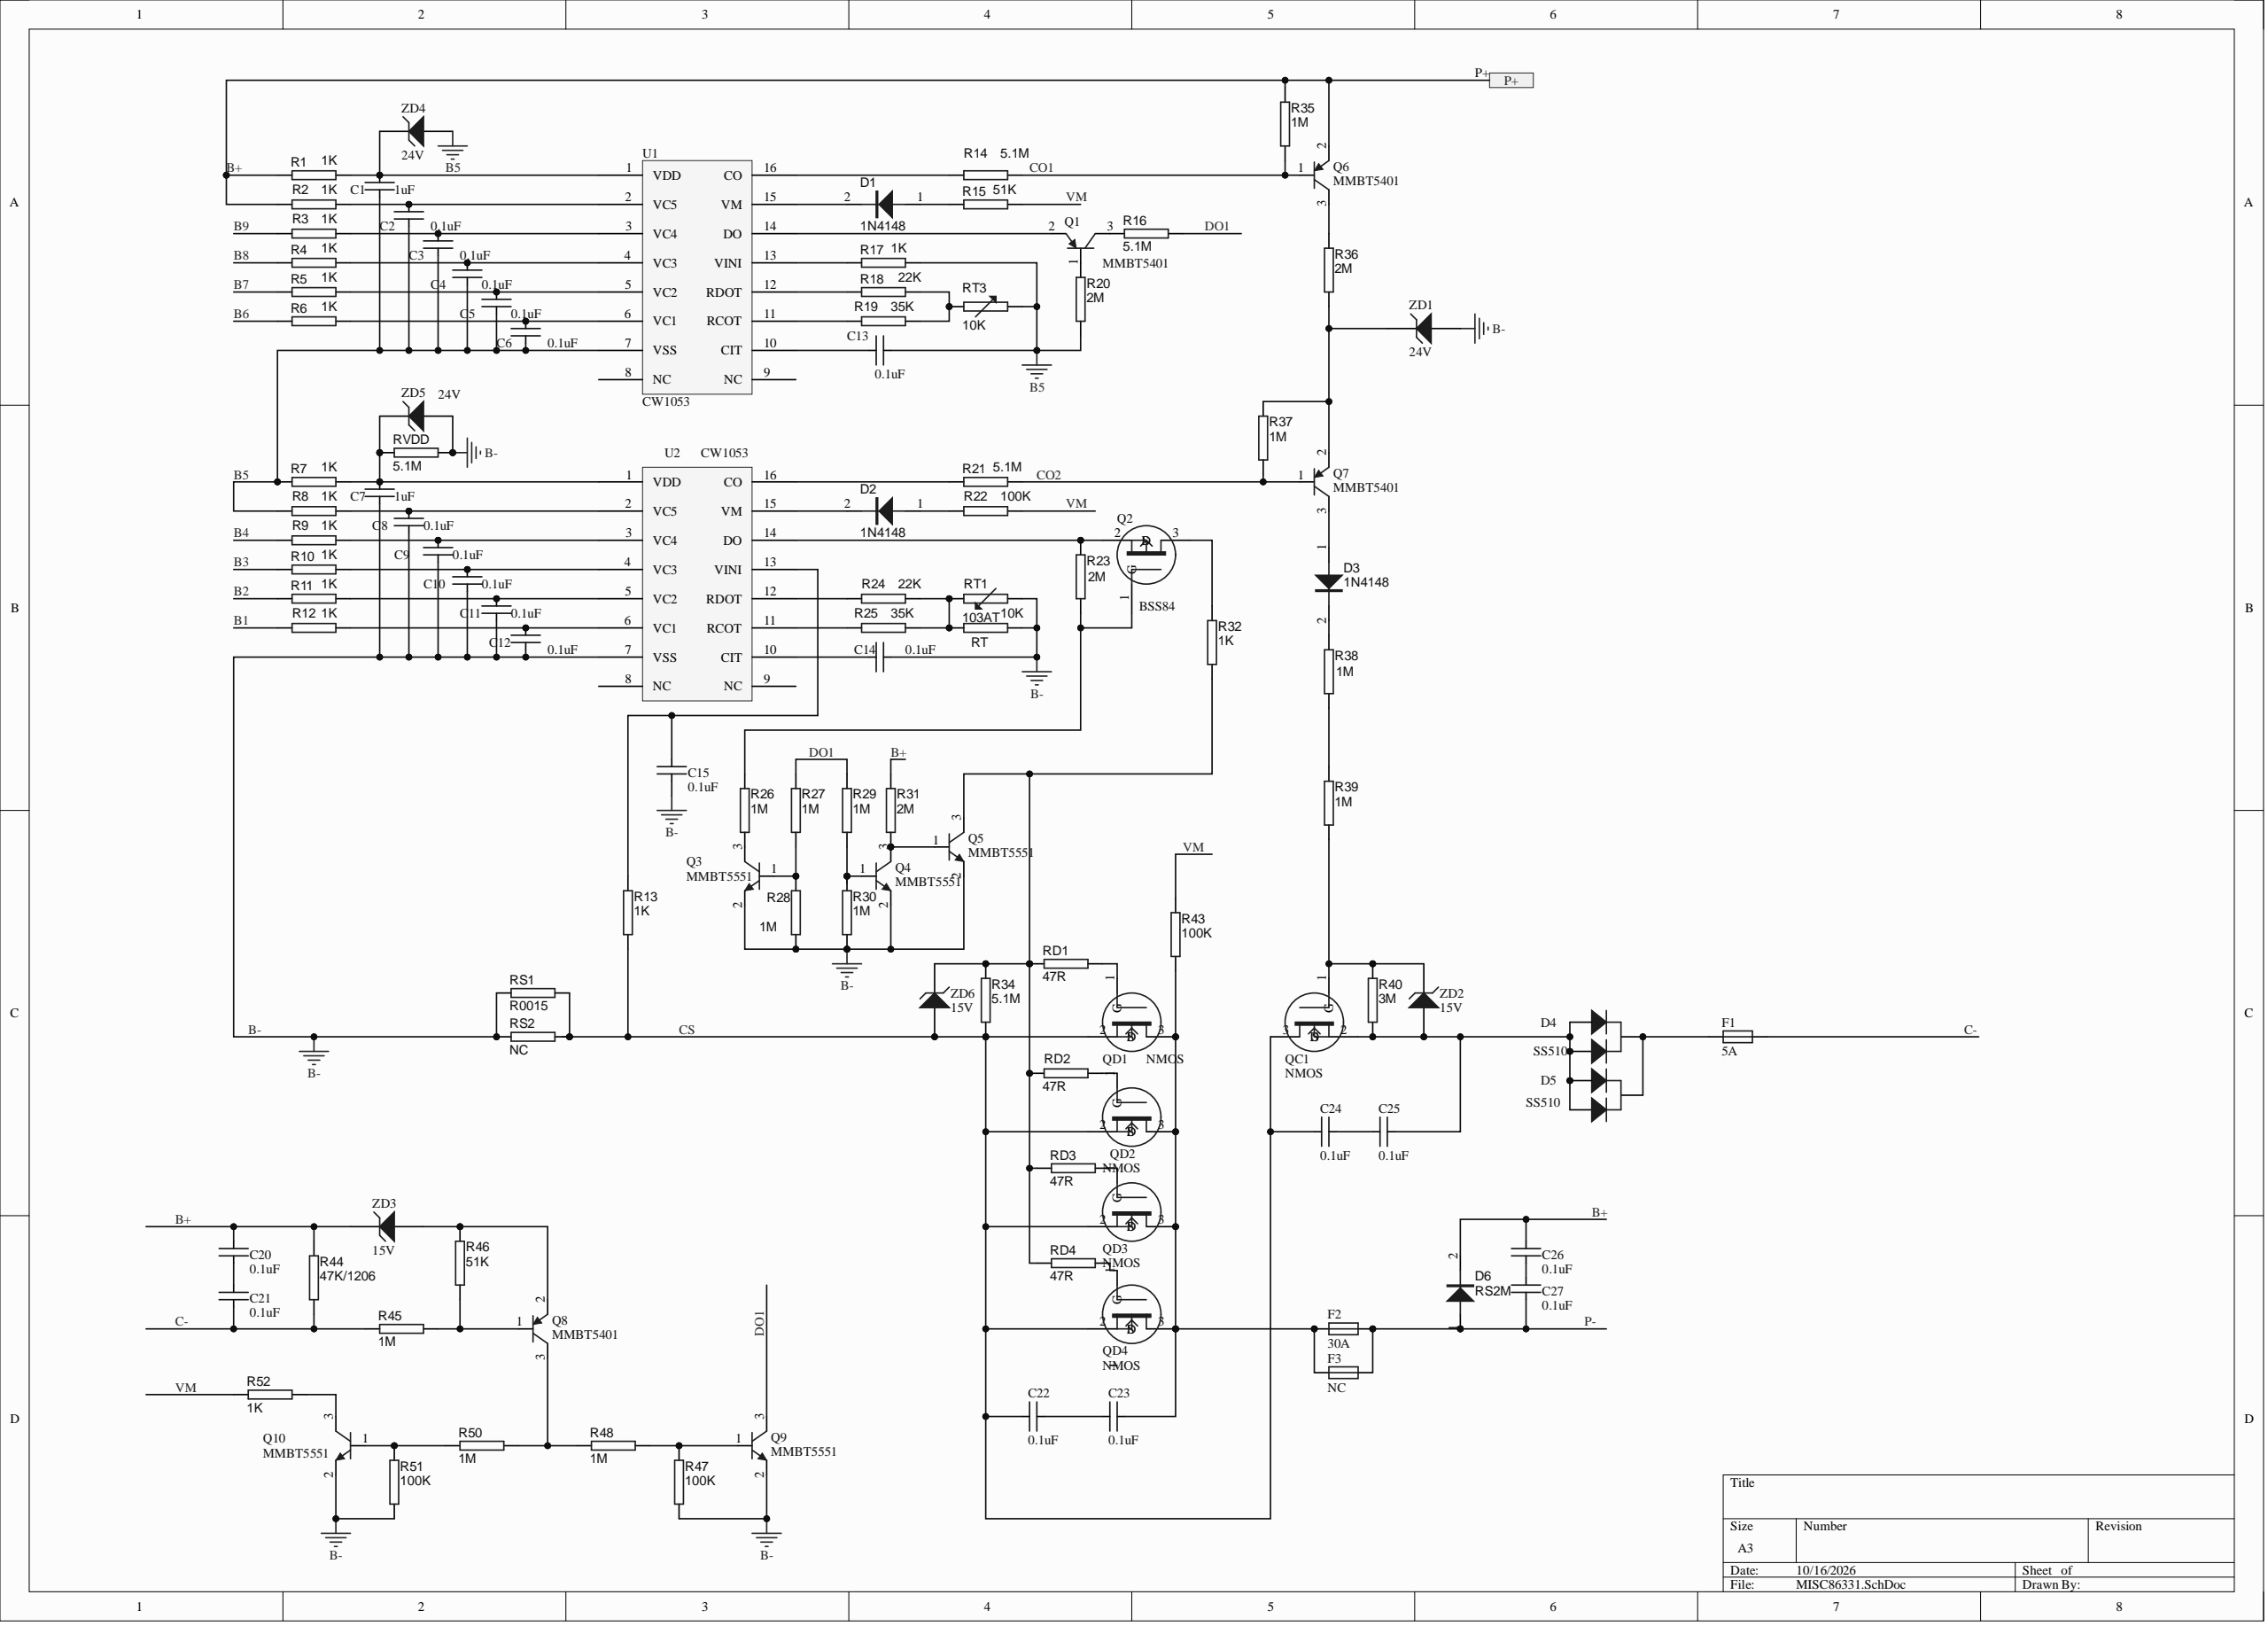Circuit board | Altium Designer | 113 parts | 72 nets
Bill of materials:
Comment,Description,Designator,Footprint,LibRef,Quantity
"1uF","CAP","C1, C7","CAP0805","CAP","2"
"0.1uF","CAP","C2, C3, C4, C5, C6, C8, C9, C10, C11, C12, C13, C14, C15, C20, C21, C22, C23, C24, C25, C26, C27","C0603A","CAP","21"
"1N4148","DIODE","D1, D2, D3","SOD323","DIODE","3"
"SS510","SMD dual common-cathode diode","D4, D5","TO-252-A","MBR10100DCT","2"
"RS2M","DIODE","D6","SMB-1","DIODE","1"
"5A","","F1","R1206","FUSE","1"
"30A","","F2","R1206","FUSE","1"
"NC","","F3","2410","FUSE","1"
"MMBT5401","PNP Bipolar Transistor","Q1, Q6, Q7, Q8","SOT-23-3","PNP","4"
"BSS84","","Q2","SOT-23-3","PMOS","1"
"MMBT5551","NPN Bipolar Transistor","Q3, Q4, Q5, Q9, Q10","SOT-23-3","NPN","5"
"NMOS","","QC1, QD1, QD2, QD3, QD4","TO-252-A","NMOS","5"
"1K","RES","R1, R7","RES0805","RES1","2"
"1K","RES","R2, R3, R4, R5, R6, R8, R9, R10, R11, R12","RES0603","RES1","10"
"1K","RES","R13, R17, R32, R52","R0603A","RES1","4"
"5.1M","RES","R14, R16, R21, R34, RVDD","R0603A","RES1","5"
"51K","RES","R15, R46","R0603A","RES1","2"
"22K","RES","R18, R24","R0603A","RES1","2"
"35K","RES","R19, R25","R0603A","RES1","2"
"2M","RES","R20, R23, R31, R36","R0603A","RES1","4"
"100K","RES","R22, R43, R47, R51","R0603A","RES1","4"
"1M","RES","R26, R27, R28, R29, R30, R35, R37, R38, R39, R45, R48, R50","R0603A","RES1","12"
"3M","RES","R40","R0603A","RES1","1"
"47K/1206","RES","R44","R1206","RES1","1"
"47R","RES","RD1, RD2, RD3, RD4","R0603A","RES1","4"
"R0015","RES","RS1","2512","RES1","1"
"NC","RES","RS2","2512","RES1","1"
"103AT","RES","RT1","WK","RES2","1"
"10K","RES","RT, RT3","R0603A","RES1, RES2","2"
"CW1053","","U1, U2","SO-16","CW1053","2"
"24V","Zener Diode","ZD1, ZD4, ZD5","SOD323","D Zener","3"
"15V","Zener Diode","ZD2, ZD3, ZD6","SOD323","D Zener","3"
Netlist (Protel format):
[
C1
CAP0805
1uF



]
[
C2
C0603A
0.1uF



]
[
C3
C0603A
0.1uF



]
[
C4
C0603A
0.1uF



]
[
C5
C0603A
0.1uF



]
[
C6
C0603A
0.1uF



]
[
C7
CAP0805
1uF



]
[
C8
C0603A
0.1uF



]
[
C9
C0603A
0.1uF



]
[
C10
C0603A
0.1uF



]
[
C11
C0603A
0.1uF



]
[
C12
C0603A
0.1uF



]
[
C13
C0603A
0.1uF



]
[
C14
C0603A
0.1uF



]
[
C15
C0603A
0.1uF



]
[
C20
C0603A
0.1uF



]
[
C21
C0603A
0.1uF



]
[
C22
C0603A
0.1uF



]
[
C23
C0603A
0.1uF



]
[
C24
C0603A
0.1uF



]
[
C25
C0603A
0.1uF



]
[
C26
C0603A
0.1uF



]
[
C27
C0603A
0.1uF



]
[
D1
SOD323
1N4148



]
[
D2
SOD323
1N4148



]
[
D3
SOD323
1N4148



]
[
D4
TO-252-A
SS510



]
[
D5
TO-252-A
SS510



]
[
D6
SMB-1
RS2M



]
[
F1
R1206
5A



]
[
F2
R1206
30A



]
[
F3
2410
NC



]
[
Q1
SOT-23-3
MMBT5401



]
[
Q2
SOT-23-3
BSS84



]
[
Q3
SOT-23-3
MMBT5551



]
[
Q4
SOT-23-3
MMBT5551



]
[
Q5
SOT-23-3
MMBT5551



]
[
Q6
SOT-23-3
MMBT5401



]
[
Q7
SOT-23-3
MMBT5401



]
[
Q8
SOT-23-3
MMBT5401



]
[
Q9
SOT-23-3
MMBT5551



]
[
Q10
SOT-23-3
MMBT5551



]
[
QC1
TO-252-A
NMOS



]
[
QD1
TO-252-A
NMOS



]
[
QD2
TO-252-A
NMOS



]
[
QD3
TO-252-A
NMOS



]
[
QD4
TO-252-A
NMOS



]
[
R1
RES0805
1K



]
[
R2
RES0603
1K



]
[
R3
RES0603
1K



]
[
R4
RES0603
1K



]
[
R5
RES0603
1K



]
[
R6
RES0603
1K



]
[
R7
RES0805
1K



]
[
R8
RES0603
1K



]
[
R9
RES0603
1K



]
[
R10
RES0603
1K



]
[
R11
RES0603
1K



]
[
R12
RES0603
1K



]
[
R13
R0603A
1K



]
[
R14
R0603A
5.1M



]
[
R15
R0603A
51K



]
[
R16
R0603A
5.1M



]
[
R17
R0603A
1K



]
[
R18
R0603A
22K



]
[
R19
R0603A
35K



]
[
R20
R0603A
2M



]
[
R21
R0603A
5.1M



]
[
R22
R0603A
100K



]
[
R23
R0603A
2M



]
[
R24
R0603A
22K



]
[
R25
R0603A
35K



]
[
R26
R0603A
1M



]
[
R27
R0603A
1M



]
[
R28
R0603A
1M



]
[
R29
R0603A
1M



]
[
R30
R0603A
1M



]
[
R31
R0603A
2M



]
[
R32
R0603A
1K



]
[
R34
R0603A
5.1M



]
[
R35
R0603A
1M



]
[
R36
R0603A
2M



]
[
R37
R0603A
1M



]
[
R38
R0603A
1M



]
[
R39
R0603A
1M



]
[
R40
R0603A
3M



]
[
R43
R0603A
100K



]
[
R44
R1206
47K/1206



]
[
R45
R0603A
1M



]
[
R46
R0603A
51K



]
[
R47
R0603A
100K



]
[
R48
R0603A
1M



]
[
R50
R0603A
1M



]
[
R51
R0603A
100K



]
[
R52
R0603A
1K



]
[
RD1
R0603A
47R



]
[
RD2
R0603A
47R



]
[
RD3
R0603A
47R



]
[
RD4
R0603A
47R



]
[
RS1
2512
R0015



]
[
RS2
2512
NC



]
[
RT
R0603A
10K



]
[
RT1
WK
103AT



]
[
RT3
R0603A
10K



]
[
RVDD
R0603A
5.1M



]
[
U1
SO-16
CW1053



]
[
U2
SO-16
CW1053



]
[
ZD1
SOD323
24V



]
[
ZD2
SOD323
15V



]
[
ZD3
SOD323
15V



]
[
ZD4
SOD323
24V



]
[
ZD5
SOD323
24V



]
[
ZD6
SOD323
15V



]
(
VM
R15-2
R22-2
R43-2
R52-1
)
(
P-
C27-1
D6-1
F2-2
F3-2
)
(
NetR38_2
R38-2
R39-2
)
(
NetR25_1
R25-1
U2-11
)
(
NetR24_2
R24-2
R25-2
RT-1
RT1-2
)
(
NetR24_1
R24-1
U2-12
)
(
NetR21_1
R21-1
U2-16
)
(
NetR19_1
R19-1
U1-11
)
(
NetR18_2
R18-2
R19-2
RT3-1
)
(
NetR18_1
R18-1
U1-12
)
(
NetR17_1
R17-1
U1-13
)
(
NetR14_1
R14-1
U1-16
)
(
NetQD4_1
QD4-1
RD4-1
)
(
NetQD3_1
QD3-1
RD3-1
)
(
NetQD2_1
QD2-1
RD2-1
)
(
NetQD1_1
QD1-1
RD1-1
)
(
NetQC1_1
QC1-1
R39-1
R40-2
ZD2-2
)
(
NetQ10_3
Q10-3
R52-2
)
(
NetQ10_1
Q10-1
R50-2
R51-1
)
(
NetQ9_1
Q9-1
R47-1
R48-1
)
(
NetQ8_3
Q8-3
R48-2
R50-1
)
(
NetQ8_2
Q8-2
R46-1
ZD3-1
)
(
NetQ8_1
Q8-1
R45-1
R46-2
)
(
NetQ7_2
Q7-2
R36-2
R37-2
ZD1-2
)
(
NetQ6_3
Q6-3
R36-1
)
(
NetQ5_3
Q5-3
R32-1
R34-2
RD1-2
RD2-2
RD3-2
RD4-2
ZD6-2
)
(
NetQ4_3
Q4-3
Q5-1
R31-1
)
(
NetQ4_1
Q4-1
R29-2
R30-2
)
(
NetQ3_3
Q3-3
R26-2
)
(
NetQ3_1
Q3-1
R27-1
R28-2
)
(
NetQ2_3
Q2-3
R32-2
)
(
NetQ2_2
Q2-2
R23-1
U2-14
)
(
NetQ2_1
Q2-1
R23-2
R26-1
)
(
NetQ1_3
Q1-3
R16-2
)
(
NetQ1_2
Q1-2
U1-14
)
(
NetQ1_1
Q1-1
R20-2
)
(
NetD4_3
D4-3
D5-3
F1-1
)
(
NetD3_2
D3-2
R38-1
)
(
NetD3_1
D3-1
Q7-3
)
(
NetD2_2
D2-2
U2-15
)
(
NetD2_1
D2-1
R22-1
)
(
NetD1_2
D1-2
U1-15
)
(
NetD1_1
D1-1
R15-1
)
(
NetC26_1
C26-1
C27-2
)
(
NetC25_1
C25-1
D4-1
D4-2
D5-1
D5-2
QC1-2
R40-1
ZD2-1
)
(
NetC24_1
C24-1
C25-2
)
(
NetC23_1
C23-1
F2-1
F3-1
QD1-3
QD2-3
QD3-3
QD4-3
R43-1
)
(
NetC22_1
C22-1
C23-2
)
(
NetC20_2
C20-2
C21-1
)
(
NetC15_2
C15-2
R13-1
U2-13
)
(
NetC14_1
C14-1
U2-10
)
(
NetC13_1
C13-1
U1-10
)
(
NetC12_1
C12-1
R12-2
U2-6
)
(
NetC11_1
C11-1
R11-1
U2-5
)
(
NetC10_1
C10-1
R10-2
U2-4
)
(
NetC9_1
C9-1
R9-2
U2-3
)
(
NetC8_1
C8-1
R8-2
U2-2
)
(
NetC7_1
C7-1
R7-2
RVDD-2
U2-1
ZD5-2
)
(
NetC6_1
C6-1
R6-2
U1-6
)
(
NetC5_1
C5-1
R5-2
U1-5
)
(
NetC4_1
C4-1
R4-2
U1-4
)
(
NetC3_1
C3-1
R3-2
U1-3
)
(
NetC2_1
C2-1
R2-2
U1-2
)
(
NetC1_1
C1-1
R1-2
U1-1
ZD4-2
)
(
DO1
Q9-3
R16-1
R27-2
R29-1
)
(
CS
C22-2
C24-2
QC1-3
QD1-2
QD2-2
QD3-2
QD4-2
R13-2
R34-1
RS1-2
RS2-2
ZD6-1
)
(
CO2
Q7-1
R21-2
R37-1
)
(
CO1
Q6-1
R14-2
R35-1
)
(
C-
C21-2
F1-2
R44-1
R45-2
)
(
B-
C7-2
C8-2
C9-2
C10-2
C11-2
C12-2
C14-2
C15-1
Q3-2
Q4-2
Q5-2
Q9-2
Q10-2
R28-1
R30-1
R47-2
R51-2
RS1-1
RS2-1
RT-2
RT1-1
RVDD-1
U2-7
ZD1-1
ZD5-1
)
(
B+
C20-1
C26-2
D6-2
Q6-2
R1-1
R2-1
R31-2
R35-2
R44-2
ZD3-2
)
(
B5
C1-2
C2-2
C3-2
C4-2
C5-2
C6-2
C13-2
R7-1
R8-1
R17-2
R20-1
RT3-2
U1-7
ZD4-1
)